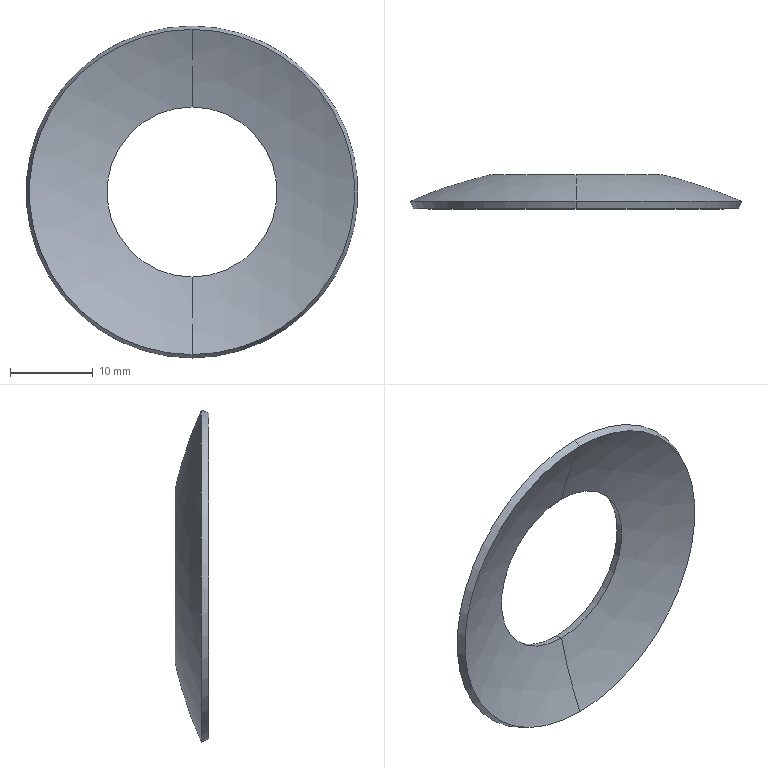Part | SolidWorks | features Revolution 1 | 1 solid | 8 faces | box 40 x 4.084 x 40 mm | volume 947.141 mm3 | cone 4 | sphere 4
STEP:
#1=CARTESIAN_POINT('',(0.,46.381,-11.75));
#2=VERTEX_POINT('',#1);
#3=CARTESIAN_POINT('',(0.,46.381,-32.25));
#4=VERTEX_POINT('',#3);
#5=CARTESIAN_POINT('',(0.,46.381,-22.));
#6=DIRECTION('',(0.,-1.,0.));
#7=DIRECTION('',(0.,0.,-1.));
#8=AXIS2_PLACEMENT_3D('',#5,#6,#7);
#9=CIRCLE('',#8,10.25);
#10=EDGE_CURVE('',#2,#4,#9,.T.);
#11=ORIENTED_EDGE('',*,*,#10,.T.);
#12=CARTESIAN_POINT('',(0.,47.357,-32.466));
#13=VERTEX_POINT('',#12);
#14=CARTESIAN_POINT('',(0.,47.357,-32.466));
#15=DIRECTION('',(0.,0.9764,-0.2158));
#16=VECTOR('',#15,1000.);
#17=LINE('',#14,#16);
#18=EDGE_CURVE('',#4,#13,#17,.T.);
#19=ORIENTED_EDGE('',*,*,#18,.T.);
#20=CARTESIAN_POINT('',(0.,47.357,-11.534));
#21=VERTEX_POINT('',#20);
#22=CARTESIAN_POINT('',(0.,47.357,-22.));
#23=DIRECTION('',(0.,-1.,0.));
#24=DIRECTION('',(0.,0.,-1.));
#25=AXIS2_PLACEMENT_3D('',#22,#23,#24);
#26=CIRCLE('',#25,10.466);
#27=EDGE_CURVE('',#21,#13,#26,.T.);
#28=ORIENTED_EDGE('',*,*,#27,.F.);
#29=CARTESIAN_POINT('',(0.,47.357,-11.534));
#30=DIRECTION('',(0.,0.9764,0.2158));
#31=VECTOR('',#30,1000.);
#32=LINE('',#29,#31);
#33=EDGE_CURVE('',#2,#21,#32,.T.);
#34=ORIENTED_EDGE('',*,*,#33,.F.);
#35=EDGE_LOOP('',(#11,#19,#28,#34));
#36=FACE_OUTER_BOUND('',#35,.T.);
#37=CARTESIAN_POINT('',(0.,47.357,-22.));
#38=DIRECTION('',(0.,1.,0.));
#39=DIRECTION('',(0.,0.,1.));
#40=AXIS2_PLACEMENT_3D('',#37,#38,#39);
#41=CONICAL_SURFACE('',#40,10.466,0.2175);
#42=ADVANCED_FACE('',(#36),#41,.F.);
#43=CARTESIAN_POINT('',(0.,47.357,-22.));
#44=DIRECTION('',(0.,-1.,0.));
#45=DIRECTION('',(0.,0.,-1.));
#46=AXIS2_PLACEMENT_3D('',#43,#44,#45);
#47=CIRCLE('',#46,10.466);
#48=EDGE_CURVE('',#13,#21,#47,.T.);
#49=ORIENTED_EDGE('',*,*,#48,.T.);
#50=CARTESIAN_POINT('',(0.,44.184,-2.));
#51=VERTEX_POINT('',#50);
#52=CARTESIAN_POINT('',(0.,0.,-22.));
#53=DIRECTION('',(1.,0.,0.));
#54=DIRECTION('',(0.,0.,-1.));
#55=AXIS2_PLACEMENT_3D('',#52,#53,#54);
#56=CIRCLE('',#55,48.5);
#57=EDGE_CURVE('',#21,#51,#56,.T.);
#58=ORIENTED_EDGE('',*,*,#57,.T.);
#59=CARTESIAN_POINT('',(0.,44.184,-42.));
#60=VERTEX_POINT('',#59);
#61=CARTESIAN_POINT('',(0.,44.184,-22.));
#62=DIRECTION('',(0.,-1.,0.));
#63=DIRECTION('',(0.,0.,-1.));
#64=AXIS2_PLACEMENT_3D('',#61,#62,#63);
#65=CIRCLE('',#64,20.);
#66=EDGE_CURVE('',#60,#51,#65,.T.);
#67=ORIENTED_EDGE('',*,*,#66,.F.);
#68=CARTESIAN_POINT('',(0.,0.,-22.));
#69=DIRECTION('',(-1.,0.,0.));
#70=DIRECTION('',(0.,0.,1.));
#71=AXIS2_PLACEMENT_3D('',#68,#69,#70);
#72=CIRCLE('',#71,48.5);
#73=EDGE_CURVE('',#13,#60,#72,.T.);
#74=ORIENTED_EDGE('',*,*,#73,.F.);
#75=EDGE_LOOP('',(#49,#58,#67,#74));
#76=FACE_OUTER_BOUND('',#75,.T.);
#77=CARTESIAN_POINT('',(0.,0.,-22.));
#78=DIRECTION('',(1.,0.,0.));
#79=DIRECTION('',(0.,0.,-1.));
#80=AXIS2_PLACEMENT_3D('',#77,#78,#79);
#81=SPHERICAL_SURFACE('',#80,48.5);
#82=ADVANCED_FACE('',(#76),#81,.T.);
#83=CARTESIAN_POINT('',(0.,43.273,-41.588));
#84=VERTEX_POINT('',#83);
#85=CARTESIAN_POINT('',(0.,43.273,-2.412));
#86=VERTEX_POINT('',#85);
#87=CARTESIAN_POINT('',(0.,43.273,-22.));
#88=DIRECTION('',(0.,-1.,0.));
#89=DIRECTION('',(0.,0.,-1.));
#90=AXIS2_PLACEMENT_3D('',#87,#88,#89);
#91=CIRCLE('',#90,19.588);
#92=EDGE_CURVE('',#84,#86,#91,.T.);
#93=ORIENTED_EDGE('',*,*,#92,.F.);
#94=CARTESIAN_POINT('',(0.,43.273,-41.588));
#95=DIRECTION('',(0.,0.911,-0.4124));
#96=VECTOR('',#95,1000.);
#97=LINE('',#94,#96);
#98=EDGE_CURVE('',#84,#60,#97,.T.);
#99=ORIENTED_EDGE('',*,*,#98,.T.);
#100=ORIENTED_EDGE('',*,*,#66,.T.);
#101=CARTESIAN_POINT('',(0.,43.273,-2.412));
#102=DIRECTION('',(0.,0.911,0.4124));
#103=VECTOR('',#102,1000.);
#104=LINE('',#101,#103);
#105=EDGE_CURVE('',#86,#51,#104,.T.);
#106=ORIENTED_EDGE('',*,*,#105,.F.);
#107=EDGE_LOOP('',(#93,#99,#100,#106));
#108=FACE_OUTER_BOUND('',#107,.T.);
#109=CARTESIAN_POINT('',(0.,43.273,-22.));
#110=DIRECTION('',(0.,1.,0.));
#111=DIRECTION('',(0.,0.,1.));
#112=AXIS2_PLACEMENT_3D('',#109,#110,#111);
#113=CONICAL_SURFACE('',#112,19.588,0.4251);
#114=ADVANCED_FACE('',(#108),#113,.T.);
#115=ORIENTED_EDGE('',*,*,#10,.F.);
#116=CARTESIAN_POINT('',(0.,0.,-22.));
#117=DIRECTION('',(1.,0.,0.));
#118=DIRECTION('',(0.,0.,-1.));
#119=AXIS2_PLACEMENT_3D('',#116,#117,#118);
#120=CIRCLE('',#119,47.5);
#121=EDGE_CURVE('',#2,#86,#120,.T.);
#122=ORIENTED_EDGE('',*,*,#121,.T.);
#123=CARTESIAN_POINT('',(0.,43.273,-22.));
#124=DIRECTION('',(0.,-1.,0.));
#125=DIRECTION('',(0.,0.,-1.));
#126=AXIS2_PLACEMENT_3D('',#123,#124,#125);
#127=CIRCLE('',#126,19.588);
#128=EDGE_CURVE('',#86,#84,#127,.T.);
#129=ORIENTED_EDGE('',*,*,#128,.T.);
#130=CARTESIAN_POINT('',(0.,0.,-22.));
#131=DIRECTION('',(-1.,0.,0.));
#132=DIRECTION('',(0.,0.,1.));
#133=AXIS2_PLACEMENT_3D('',#130,#131,#132);
#134=CIRCLE('',#133,47.5);
#135=EDGE_CURVE('',#4,#84,#134,.T.);
#136=ORIENTED_EDGE('',*,*,#135,.F.);
#137=EDGE_LOOP('',(#115,#122,#129,#136));
#138=FACE_OUTER_BOUND('',#137,.T.);
#139=CARTESIAN_POINT('',(0.,0.,-22.));
#140=DIRECTION('',(1.,0.,0.));
#141=DIRECTION('',(0.,0.,-1.));
#142=AXIS2_PLACEMENT_3D('',#139,#140,#141);
#143=SPHERICAL_SURFACE('',#142,47.5);
#144=ADVANCED_FACE('',(#138),#143,.F.);
#145=ORIENTED_EDGE('',*,*,#121,.F.);
#146=CARTESIAN_POINT('',(0.,46.381,-22.));
#147=DIRECTION('',(0.,-1.,0.));
#148=DIRECTION('',(0.,0.,-1.));
#149=AXIS2_PLACEMENT_3D('',#146,#147,#148);
#150=CIRCLE('',#149,10.25);
#151=EDGE_CURVE('',#4,#2,#150,.T.);
#152=ORIENTED_EDGE('',*,*,#151,.F.);
#153=ORIENTED_EDGE('',*,*,#135,.T.);
#154=ORIENTED_EDGE('',*,*,#92,.T.);
#155=EDGE_LOOP('',(#145,#152,#153,#154));
#156=FACE_OUTER_BOUND('',#155,.T.);
#157=CARTESIAN_POINT('',(0.,0.,-22.));
#158=DIRECTION('',(1.,0.,0.));
#159=DIRECTION('',(0.,0.,-1.));
#160=AXIS2_PLACEMENT_3D('',#157,#158,#159);
#161=SPHERICAL_SURFACE('',#160,47.5);
#162=ADVANCED_FACE('',(#156),#161,.F.);
#163=ORIENTED_EDGE('',*,*,#98,.F.);
#164=ORIENTED_EDGE('',*,*,#128,.F.);
#165=ORIENTED_EDGE('',*,*,#105,.T.);
#166=CARTESIAN_POINT('',(0.,44.184,-22.));
#167=DIRECTION('',(0.,-1.,0.));
#168=DIRECTION('',(0.,0.,-1.));
#169=AXIS2_PLACEMENT_3D('',#166,#167,#168);
#170=CIRCLE('',#169,20.);
#171=EDGE_CURVE('',#51,#60,#170,.T.);
#172=ORIENTED_EDGE('',*,*,#171,.T.);
#173=EDGE_LOOP('',(#163,#164,#165,#172));
#174=FACE_OUTER_BOUND('',#173,.T.);
#175=CARTESIAN_POINT('',(0.,43.273,-22.));
#176=DIRECTION('',(0.,1.,0.));
#177=DIRECTION('',(0.,0.,1.));
#178=AXIS2_PLACEMENT_3D('',#175,#176,#177);
#179=CONICAL_SURFACE('',#178,19.588,0.4251);
#180=ADVANCED_FACE('',(#174),#179,.T.);
#181=ORIENTED_EDGE('',*,*,#57,.F.);
#182=ORIENTED_EDGE('',*,*,#27,.T.);
#183=ORIENTED_EDGE('',*,*,#73,.T.);
#184=ORIENTED_EDGE('',*,*,#171,.F.);
#185=EDGE_LOOP('',(#181,#182,#183,#184));
#186=FACE_OUTER_BOUND('',#185,.T.);
#187=CARTESIAN_POINT('',(0.,0.,-22.));
#188=DIRECTION('',(1.,0.,0.));
#189=DIRECTION('',(0.,0.,-1.));
#190=AXIS2_PLACEMENT_3D('',#187,#188,#189);
#191=SPHERICAL_SURFACE('',#190,48.5);
#192=ADVANCED_FACE('',(#186),#191,.T.);
#193=ORIENTED_EDGE('',*,*,#18,.F.);
#194=ORIENTED_EDGE('',*,*,#151,.T.);
#195=ORIENTED_EDGE('',*,*,#33,.T.);
#196=ORIENTED_EDGE('',*,*,#48,.F.);
#197=EDGE_LOOP('',(#193,#194,#195,#196));
#198=FACE_OUTER_BOUND('',#197,.T.);
#199=CARTESIAN_POINT('',(0.,47.357,-22.));
#200=DIRECTION('',(0.,1.,0.));
#201=DIRECTION('',(0.,0.,1.));
#202=AXIS2_PLACEMENT_3D('',#199,#200,#201);
#203=CONICAL_SURFACE('',#202,10.466,0.2175);
#204=ADVANCED_FACE('',(#198),#203,.F.);
#205=CLOSED_SHELL('',(#42,#82,#114,#144,#162,#180,#192,#204));
#206=MANIFOLD_SOLID_BREP('',#205);
#207=CARTESIAN_POINT('',(0.,0.,0.));
#208=DIRECTION('',(0.,0.,1.));
#209=DIRECTION('',(1.,0.,0.));
#210=AXIS2_PLACEMENT_3D('',#207,#208,#209);
#211=(LENGTH_UNIT()NAMED_UNIT(*)SI_UNIT(.MILLI.,.METRE.));
#212=UNCERTAINTY_MEASURE_WITH_UNIT(LENGTH_MEASURE(0.00001),#211,'','');
#213=(NAMED_UNIT(*)PLANE_ANGLE_UNIT()SI_UNIT($,.RADIAN.));
#214=(NAMED_UNIT(*)SI_UNIT($,.STERADIAN.)SOLID_ANGLE_UNIT());
#215=(GEOMETRIC_REPRESENTATION_CONTEXT(3)GLOBAL_UNCERTAINTY_ASSIGNED_CONTEXT((#212))GLOBAL_UNIT_ASSIGNED_CONTEXT((#211,#213,#214))REPRESENTATION_CONTEXT('',''));
#216=ADVANCED_BREP_SHAPE_REPRESENTATION('',(#206,#210),#215);